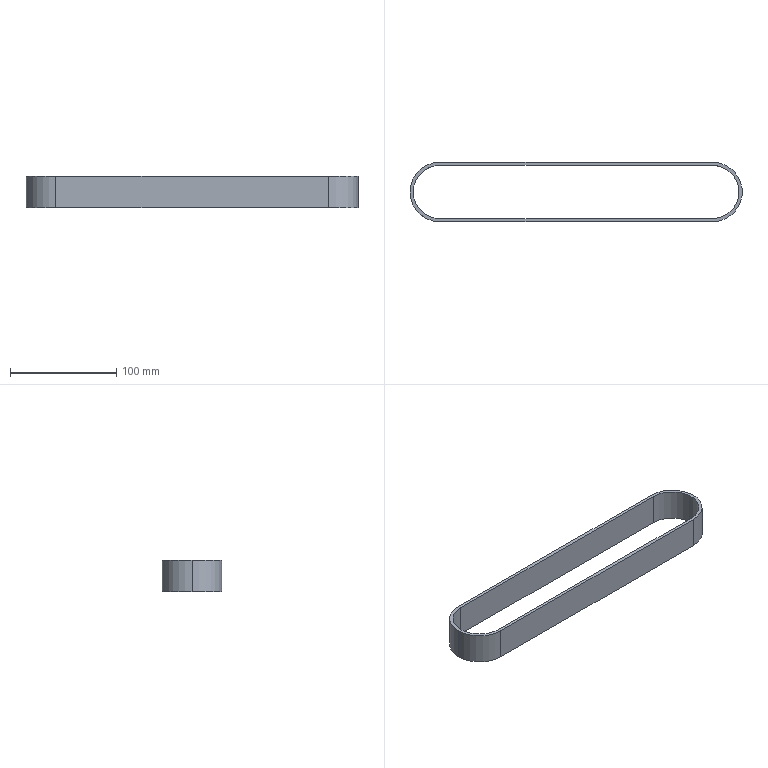Part | SolidWorks | features ExtruThin 1 | 1 solid | 12 faces | box 312 x 56 x 30 mm | volume 61065 mm3 | cylinder 6 | plane 6 | commonest cylinder face diameters 50 x3 56 x3
STEP:
#1=CARTESIAN_POINT('',(-128.,25.,30.));
#2=VERTEX_POINT('',#1);
#3=CARTESIAN_POINT('',(-153.,0.,30.));
#4=VERTEX_POINT('',#3);
#5=CARTESIAN_POINT('',(-128.,0.,30.));
#6=DIRECTION('',(0.,0.,1.));
#7=DIRECTION('',(1.,0.,0.));
#8=AXIS2_PLACEMENT_3D('',#5,#6,#7);
#9=CIRCLE('',#8,25.);
#10=EDGE_CURVE('',#2,#4,#9,.T.);
#11=ORIENTED_EDGE('',*,*,#10,.T.);
#12=CARTESIAN_POINT('',(-153.,0.,0.));
#13=VERTEX_POINT('',#12);
#14=CARTESIAN_POINT('',(-153.,0.,30.));
#15=DIRECTION('',(0.,0.,-1.));
#16=VECTOR('',#15,1000.);
#17=LINE('',#14,#16);
#18=EDGE_CURVE('',#4,#13,#17,.T.);
#19=ORIENTED_EDGE('',*,*,#18,.T.);
#20=CARTESIAN_POINT('',(-128.,25.,0.));
#21=VERTEX_POINT('',#20);
#22=CARTESIAN_POINT('',(-128.,0.,0.));
#23=DIRECTION('',(0.,0.,1.));
#24=DIRECTION('',(1.,0.,0.));
#25=AXIS2_PLACEMENT_3D('',#22,#23,#24);
#26=CIRCLE('',#25,25.);
#27=EDGE_CURVE('',#21,#13,#26,.T.);
#28=ORIENTED_EDGE('',*,*,#27,.F.);
#29=CARTESIAN_POINT('',(-128.,25.,30.));
#30=DIRECTION('',(0.,0.,-1.));
#31=VECTOR('',#30,1000.);
#32=LINE('',#29,#31);
#33=EDGE_CURVE('',#2,#21,#32,.T.);
#34=ORIENTED_EDGE('',*,*,#33,.F.);
#35=EDGE_LOOP('',(#11,#19,#28,#34));
#36=FACE_OUTER_BOUND('',#35,.T.);
#37=CARTESIAN_POINT('',(-128.,0.,30.));
#38=DIRECTION('',(0.,0.,-1.));
#39=DIRECTION('',(-1.,0.,0.));
#40=AXIS2_PLACEMENT_3D('',#37,#38,#39);
#41=CYLINDRICAL_SURFACE('',#40,25.);
#42=ADVANCED_FACE('',(#36),#41,.F.);
#43=CARTESIAN_POINT('',(-156.,0.,30.));
#44=VERTEX_POINT('',#43);
#45=CARTESIAN_POINT('',(-128.,-28.,30.));
#46=VERTEX_POINT('',#45);
#47=CARTESIAN_POINT('',(-128.,0.,30.));
#48=DIRECTION('',(0.,0.,1.));
#49=DIRECTION('',(1.,0.,0.));
#50=AXIS2_PLACEMENT_3D('',#47,#48,#49);
#51=CIRCLE('',#50,28.);
#52=EDGE_CURVE('',#44,#46,#51,.T.);
#53=ORIENTED_EDGE('',*,*,#52,.F.);
#54=CARTESIAN_POINT('',(-156.,0.,0.));
#55=VERTEX_POINT('',#54);
#56=CARTESIAN_POINT('',(-156.,0.,30.));
#57=DIRECTION('',(0.,0.,-1.));
#58=VECTOR('',#57,1000.);
#59=LINE('',#56,#58);
#60=EDGE_CURVE('',#44,#55,#59,.T.);
#61=ORIENTED_EDGE('',*,*,#60,.T.);
#62=CARTESIAN_POINT('',(-128.,-28.,0.));
#63=VERTEX_POINT('',#62);
#64=CARTESIAN_POINT('',(-128.,0.,0.));
#65=DIRECTION('',(0.,0.,1.));
#66=DIRECTION('',(1.,0.,0.));
#67=AXIS2_PLACEMENT_3D('',#64,#65,#66);
#68=CIRCLE('',#67,28.);
#69=EDGE_CURVE('',#55,#63,#68,.T.);
#70=ORIENTED_EDGE('',*,*,#69,.T.);
#71=CARTESIAN_POINT('',(-128.,-28.,30.));
#72=DIRECTION('',(0.,0.,-1.));
#73=VECTOR('',#72,1000.);
#74=LINE('',#71,#73);
#75=EDGE_CURVE('',#46,#63,#74,.T.);
#76=ORIENTED_EDGE('',*,*,#75,.F.);
#77=EDGE_LOOP('',(#53,#61,#70,#76));
#78=FACE_OUTER_BOUND('',#77,.T.);
#79=CARTESIAN_POINT('',(-128.,0.,30.));
#80=DIRECTION('',(0.,0.,-1.));
#81=DIRECTION('',(-1.,0.,0.));
#82=AXIS2_PLACEMENT_3D('',#79,#80,#81);
#83=CYLINDRICAL_SURFACE('',#82,28.);
#84=ADVANCED_FACE('',(#78),#83,.T.);
#85=CARTESIAN_POINT('',(-128.,28.,30.));
#86=VERTEX_POINT('',#85);
#87=CARTESIAN_POINT('',(-128.,0.,30.));
#88=DIRECTION('',(0.,0.,1.));
#89=DIRECTION('',(1.,0.,0.));
#90=AXIS2_PLACEMENT_3D('',#87,#88,#89);
#91=CIRCLE('',#90,28.);
#92=EDGE_CURVE('',#86,#44,#91,.T.);
#93=ORIENTED_EDGE('',*,*,#92,.T.);
#94=ORIENTED_EDGE('',*,*,#52,.T.);
#95=CARTESIAN_POINT('',(128.,-28.,30.));
#96=VERTEX_POINT('',#95);
#97=CARTESIAN_POINT('',(-128.,-28.,30.));
#98=DIRECTION('',(1.,0.,0.));
#99=VECTOR('',#98,1000.);
#100=LINE('',#97,#99);
#101=EDGE_CURVE('',#46,#96,#100,.T.);
#102=ORIENTED_EDGE('',*,*,#101,.T.);
#103=CARTESIAN_POINT('',(128.,28.,30.));
#104=VERTEX_POINT('',#103);
#105=CARTESIAN_POINT('',(128.,0.,30.));
#106=DIRECTION('',(0.,0.,1.));
#107=DIRECTION('',(1.,0.,0.));
#108=AXIS2_PLACEMENT_3D('',#105,#106,#107);
#109=CIRCLE('',#108,28.);
#110=EDGE_CURVE('',#96,#104,#109,.T.);
#111=ORIENTED_EDGE('',*,*,#110,.T.);
#112=CARTESIAN_POINT('',(-128.,28.,30.));
#113=DIRECTION('',(-1.,0.,0.));
#114=VECTOR('',#113,1000.);
#115=LINE('',#112,#114);
#116=EDGE_CURVE('',#104,#86,#115,.T.);
#117=ORIENTED_EDGE('',*,*,#116,.T.);
#118=EDGE_LOOP('',(#93,#94,#102,#111,#117));
#119=FACE_OUTER_BOUND('',#118,.T.);
#120=CARTESIAN_POINT('',(-128.,-25.,30.));
#121=VERTEX_POINT('',#120);
#122=CARTESIAN_POINT('',(128.,-25.,30.));
#123=VERTEX_POINT('',#122);
#124=CARTESIAN_POINT('',(-128.,-25.,30.));
#125=DIRECTION('',(1.,0.,0.));
#126=VECTOR('',#125,1000.);
#127=LINE('',#124,#126);
#128=EDGE_CURVE('',#121,#123,#127,.T.);
#129=ORIENTED_EDGE('',*,*,#128,.F.);
#130=CARTESIAN_POINT('',(-128.,0.,30.));
#131=DIRECTION('',(0.,0.,1.));
#132=DIRECTION('',(1.,0.,0.));
#133=AXIS2_PLACEMENT_3D('',#130,#131,#132);
#134=CIRCLE('',#133,25.);
#135=EDGE_CURVE('',#4,#121,#134,.T.);
#136=ORIENTED_EDGE('',*,*,#135,.F.);
#137=ORIENTED_EDGE('',*,*,#10,.F.);
#138=CARTESIAN_POINT('',(128.,25.,30.));
#139=VERTEX_POINT('',#138);
#140=CARTESIAN_POINT('',(-128.,25.,30.));
#141=DIRECTION('',(-1.,0.,0.));
#142=VECTOR('',#141,1000.);
#143=LINE('',#140,#142);
#144=EDGE_CURVE('',#139,#2,#143,.T.);
#145=ORIENTED_EDGE('',*,*,#144,.F.);
#146=CARTESIAN_POINT('',(128.,0.,30.));
#147=DIRECTION('',(0.,0.,1.));
#148=DIRECTION('',(1.,0.,0.));
#149=AXIS2_PLACEMENT_3D('',#146,#147,#148);
#150=CIRCLE('',#149,25.);
#151=EDGE_CURVE('',#123,#139,#150,.T.);
#152=ORIENTED_EDGE('',*,*,#151,.F.);
#153=EDGE_LOOP('',(#129,#136,#137,#145,#152));
#154=FACE_BOUND('',#153,.T.);
#155=CARTESIAN_POINT('',(-128.,0.,30.));
#156=DIRECTION('',(0.,0.,1.));
#157=DIRECTION('',(1.,0.,0.));
#158=AXIS2_PLACEMENT_3D('',#155,#156,#157);
#159=PLANE('',#158);
#160=ADVANCED_FACE('',(#119,#154),#159,.T.);
#161=CARTESIAN_POINT('',(-128.,28.,0.));
#162=VERTEX_POINT('',#161);
#163=CARTESIAN_POINT('',(-128.,0.,0.));
#164=DIRECTION('',(0.,0.,1.));
#165=DIRECTION('',(1.,0.,0.));
#166=AXIS2_PLACEMENT_3D('',#163,#164,#165);
#167=CIRCLE('',#166,28.);
#168=EDGE_CURVE('',#162,#55,#167,.T.);
#169=ORIENTED_EDGE('',*,*,#168,.F.);
#170=CARTESIAN_POINT('',(128.,28.,0.));
#171=VERTEX_POINT('',#170);
#172=CARTESIAN_POINT('',(-128.,28.,0.));
#173=DIRECTION('',(-1.,0.,0.));
#174=VECTOR('',#173,1000.);
#175=LINE('',#172,#174);
#176=EDGE_CURVE('',#171,#162,#175,.T.);
#177=ORIENTED_EDGE('',*,*,#176,.F.);
#178=CARTESIAN_POINT('',(128.,-28.,0.));
#179=VERTEX_POINT('',#178);
#180=CARTESIAN_POINT('',(128.,0.,0.));
#181=DIRECTION('',(0.,0.,1.));
#182=DIRECTION('',(1.,0.,0.));
#183=AXIS2_PLACEMENT_3D('',#180,#181,#182);
#184=CIRCLE('',#183,28.);
#185=EDGE_CURVE('',#179,#171,#184,.T.);
#186=ORIENTED_EDGE('',*,*,#185,.F.);
#187=CARTESIAN_POINT('',(-128.,-28.,0.));
#188=DIRECTION('',(1.,0.,0.));
#189=VECTOR('',#188,1000.);
#190=LINE('',#187,#189);
#191=EDGE_CURVE('',#63,#179,#190,.T.);
#192=ORIENTED_EDGE('',*,*,#191,.F.);
#193=ORIENTED_EDGE('',*,*,#69,.F.);
#194=EDGE_LOOP('',(#169,#177,#186,#192,#193));
#195=FACE_OUTER_BOUND('',#194,.T.);
#196=ORIENTED_EDGE('',*,*,#27,.T.);
#197=CARTESIAN_POINT('',(-128.,-25.,0.));
#198=VERTEX_POINT('',#197);
#199=CARTESIAN_POINT('',(-128.,0.,0.));
#200=DIRECTION('',(0.,0.,1.));
#201=DIRECTION('',(1.,0.,0.));
#202=AXIS2_PLACEMENT_3D('',#199,#200,#201);
#203=CIRCLE('',#202,25.);
#204=EDGE_CURVE('',#13,#198,#203,.T.);
#205=ORIENTED_EDGE('',*,*,#204,.T.);
#206=CARTESIAN_POINT('',(128.,-25.,0.));
#207=VERTEX_POINT('',#206);
#208=CARTESIAN_POINT('',(-128.,-25.,0.));
#209=DIRECTION('',(1.,0.,0.));
#210=VECTOR('',#209,1000.);
#211=LINE('',#208,#210);
#212=EDGE_CURVE('',#198,#207,#211,.T.);
#213=ORIENTED_EDGE('',*,*,#212,.T.);
#214=CARTESIAN_POINT('',(128.,25.,0.));
#215=VERTEX_POINT('',#214);
#216=CARTESIAN_POINT('',(128.,0.,0.));
#217=DIRECTION('',(0.,0.,1.));
#218=DIRECTION('',(1.,0.,0.));
#219=AXIS2_PLACEMENT_3D('',#216,#217,#218);
#220=CIRCLE('',#219,25.);
#221=EDGE_CURVE('',#207,#215,#220,.T.);
#222=ORIENTED_EDGE('',*,*,#221,.T.);
#223=CARTESIAN_POINT('',(-128.,25.,0.));
#224=DIRECTION('',(-1.,0.,0.));
#225=VECTOR('',#224,1000.);
#226=LINE('',#223,#225);
#227=EDGE_CURVE('',#215,#21,#226,.T.);
#228=ORIENTED_EDGE('',*,*,#227,.T.);
#229=EDGE_LOOP('',(#196,#205,#213,#222,#228));
#230=FACE_BOUND('',#229,.T.);
#231=CARTESIAN_POINT('',(-128.,0.,0.));
#232=DIRECTION('',(0.,0.,1.));
#233=DIRECTION('',(1.,0.,0.));
#234=AXIS2_PLACEMENT_3D('',#231,#232,#233);
#235=PLANE('',#234);
#236=ADVANCED_FACE('',(#195,#230),#235,.F.);
#237=ORIENTED_EDGE('',*,*,#60,.F.);
#238=ORIENTED_EDGE('',*,*,#92,.F.);
#239=CARTESIAN_POINT('',(-128.,28.,30.));
#240=DIRECTION('',(0.,0.,-1.));
#241=VECTOR('',#240,1000.);
#242=LINE('',#239,#241);
#243=EDGE_CURVE('',#86,#162,#242,.T.);
#244=ORIENTED_EDGE('',*,*,#243,.T.);
#245=ORIENTED_EDGE('',*,*,#168,.T.);
#246=EDGE_LOOP('',(#237,#238,#244,#245));
#247=FACE_OUTER_BOUND('',#246,.T.);
#248=CARTESIAN_POINT('',(-128.,0.,30.));
#249=DIRECTION('',(0.,0.,-1.));
#250=DIRECTION('',(-1.,0.,0.));
#251=AXIS2_PLACEMENT_3D('',#248,#249,#250);
#252=CYLINDRICAL_SURFACE('',#251,28.);
#253=ADVANCED_FACE('',(#247),#252,.T.);
#254=ORIENTED_EDGE('',*,*,#191,.T.);
#255=CARTESIAN_POINT('',(128.,-28.,30.));
#256=DIRECTION('',(0.,0.,-1.));
#257=VECTOR('',#256,1000.);
#258=LINE('',#255,#257);
#259=EDGE_CURVE('',#96,#179,#258,.T.);
#260=ORIENTED_EDGE('',*,*,#259,.F.);
#261=ORIENTED_EDGE('',*,*,#101,.F.);
#262=ORIENTED_EDGE('',*,*,#75,.T.);
#263=EDGE_LOOP('',(#254,#260,#261,#262));
#264=FACE_OUTER_BOUND('',#263,.T.);
#265=CARTESIAN_POINT('',(-128.,-28.,30.));
#266=DIRECTION('',(0.,1.,0.));
#267=DIRECTION('',(0.,0.,1.));
#268=AXIS2_PLACEMENT_3D('',#265,#266,#267);
#269=PLANE('',#268);
#270=ADVANCED_FACE('',(#264),#269,.F.);
#271=ORIENTED_EDGE('',*,*,#185,.T.);
#272=CARTESIAN_POINT('',(128.,28.,30.));
#273=DIRECTION('',(0.,0.,-1.));
#274=VECTOR('',#273,1000.);
#275=LINE('',#272,#274);
#276=EDGE_CURVE('',#104,#171,#275,.T.);
#277=ORIENTED_EDGE('',*,*,#276,.F.);
#278=ORIENTED_EDGE('',*,*,#110,.F.);
#279=ORIENTED_EDGE('',*,*,#259,.T.);
#280=EDGE_LOOP('',(#271,#277,#278,#279));
#281=FACE_OUTER_BOUND('',#280,.T.);
#282=CARTESIAN_POINT('',(128.,0.,30.));
#283=DIRECTION('',(0.,0.,-1.));
#284=DIRECTION('',(-1.,0.,0.));
#285=AXIS2_PLACEMENT_3D('',#282,#283,#284);
#286=CYLINDRICAL_SURFACE('',#285,28.);
#287=ADVANCED_FACE('',(#281),#286,.T.);
#288=ORIENTED_EDGE('',*,*,#176,.T.);
#289=ORIENTED_EDGE('',*,*,#243,.F.);
#290=ORIENTED_EDGE('',*,*,#116,.F.);
#291=ORIENTED_EDGE('',*,*,#276,.T.);
#292=EDGE_LOOP('',(#288,#289,#290,#291));
#293=FACE_OUTER_BOUND('',#292,.T.);
#294=CARTESIAN_POINT('',(-128.,28.,30.));
#295=DIRECTION('',(0.,-1.,0.));
#296=DIRECTION('',(0.,0.,-1.));
#297=AXIS2_PLACEMENT_3D('',#294,#295,#296);
#298=PLANE('',#297);
#299=ADVANCED_FACE('',(#293),#298,.F.);
#300=ORIENTED_EDGE('',*,*,#18,.F.);
#301=ORIENTED_EDGE('',*,*,#135,.T.);
#302=CARTESIAN_POINT('',(-128.,-25.,30.));
#303=DIRECTION('',(0.,0.,-1.));
#304=VECTOR('',#303,1000.);
#305=LINE('',#302,#304);
#306=EDGE_CURVE('',#121,#198,#305,.T.);
#307=ORIENTED_EDGE('',*,*,#306,.T.);
#308=ORIENTED_EDGE('',*,*,#204,.F.);
#309=EDGE_LOOP('',(#300,#301,#307,#308));
#310=FACE_OUTER_BOUND('',#309,.T.);
#311=CARTESIAN_POINT('',(-128.,0.,30.));
#312=DIRECTION('',(0.,0.,-1.));
#313=DIRECTION('',(-1.,0.,0.));
#314=AXIS2_PLACEMENT_3D('',#311,#312,#313);
#315=CYLINDRICAL_SURFACE('',#314,25.);
#316=ADVANCED_FACE('',(#310),#315,.F.);
#317=ORIENTED_EDGE('',*,*,#212,.F.);
#318=ORIENTED_EDGE('',*,*,#306,.F.);
#319=ORIENTED_EDGE('',*,*,#128,.T.);
#320=CARTESIAN_POINT('',(128.,-25.,30.));
#321=DIRECTION('',(0.,0.,-1.));
#322=VECTOR('',#321,1000.);
#323=LINE('',#320,#322);
#324=EDGE_CURVE('',#123,#207,#323,.T.);
#325=ORIENTED_EDGE('',*,*,#324,.T.);
#326=EDGE_LOOP('',(#317,#318,#319,#325));
#327=FACE_OUTER_BOUND('',#326,.T.);
#328=CARTESIAN_POINT('',(-128.,-25.,30.));
#329=DIRECTION('',(0.,1.,0.));
#330=DIRECTION('',(0.,0.,1.));
#331=AXIS2_PLACEMENT_3D('',#328,#329,#330);
#332=PLANE('',#331);
#333=ADVANCED_FACE('',(#327),#332,.T.);
#334=ORIENTED_EDGE('',*,*,#221,.F.);
#335=ORIENTED_EDGE('',*,*,#324,.F.);
#336=ORIENTED_EDGE('',*,*,#151,.T.);
#337=CARTESIAN_POINT('',(128.,25.,30.));
#338=DIRECTION('',(0.,0.,-1.));
#339=VECTOR('',#338,1000.);
#340=LINE('',#337,#339);
#341=EDGE_CURVE('',#139,#215,#340,.T.);
#342=ORIENTED_EDGE('',*,*,#341,.T.);
#343=EDGE_LOOP('',(#334,#335,#336,#342));
#344=FACE_OUTER_BOUND('',#343,.T.);
#345=CARTESIAN_POINT('',(128.,0.,30.));
#346=DIRECTION('',(0.,0.,-1.));
#347=DIRECTION('',(-1.,0.,0.));
#348=AXIS2_PLACEMENT_3D('',#345,#346,#347);
#349=CYLINDRICAL_SURFACE('',#348,25.);
#350=ADVANCED_FACE('',(#344),#349,.F.);
#351=ORIENTED_EDGE('',*,*,#227,.F.);
#352=ORIENTED_EDGE('',*,*,#341,.F.);
#353=ORIENTED_EDGE('',*,*,#144,.T.);
#354=ORIENTED_EDGE('',*,*,#33,.T.);
#355=EDGE_LOOP('',(#351,#352,#353,#354));
#356=FACE_OUTER_BOUND('',#355,.T.);
#357=CARTESIAN_POINT('',(-128.,25.,30.));
#358=DIRECTION('',(0.,-1.,0.));
#359=DIRECTION('',(0.,0.,-1.));
#360=AXIS2_PLACEMENT_3D('',#357,#358,#359);
#361=PLANE('',#360);
#362=ADVANCED_FACE('',(#356),#361,.T.);
#363=CLOSED_SHELL('',(#42,#84,#160,#236,#253,#270,#287,#299,#316,#333,#350,#362));
#364=MANIFOLD_SOLID_BREP('',#363);
#365=CARTESIAN_POINT('',(0.,0.,0.));
#366=DIRECTION('',(0.,0.,1.));
#367=DIRECTION('',(1.,0.,0.));
#368=AXIS2_PLACEMENT_3D('',#365,#366,#367);
#369=(LENGTH_UNIT()NAMED_UNIT(*)SI_UNIT(.MILLI.,.METRE.));
#370=UNCERTAINTY_MEASURE_WITH_UNIT(LENGTH_MEASURE(0.00001),#369,'','');
#371=(NAMED_UNIT(*)PLANE_ANGLE_UNIT()SI_UNIT($,.RADIAN.));
#372=(NAMED_UNIT(*)SI_UNIT($,.STERADIAN.)SOLID_ANGLE_UNIT());
#373=(GEOMETRIC_REPRESENTATION_CONTEXT(3)GLOBAL_UNCERTAINTY_ASSIGNED_CONTEXT((#370))GLOBAL_UNIT_ASSIGNED_CONTEXT((#369,#371,#372))REPRESENTATION_CONTEXT('',''));
#374=ADVANCED_BREP_SHAPE_REPRESENTATION('',(#364,#368),#373);